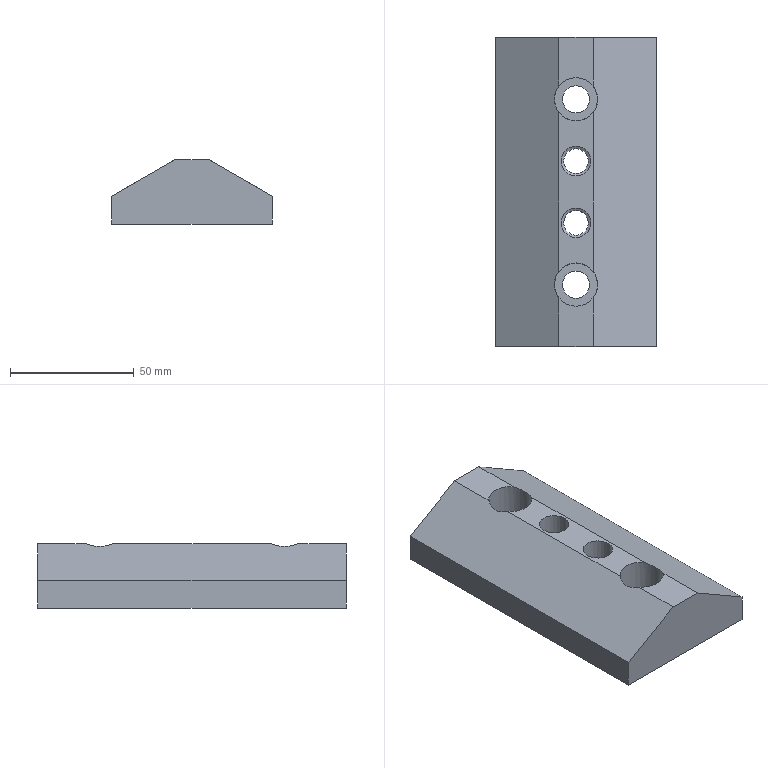Part | NX | features MAIN_BODY 2 | 1 solid | 22 faces | box 65 x 125 x 26 mm | volume 149619 mm3 | plane 12 | cylinder 8 | cone 2 | commonest cylinder face diameters 10 x2 11 x2 12 x2 17.5 x2
STEP:
#1=CARTESIAN_POINT('',(418.072,449.656,-244.));
#2=VERTEX_POINT('',#1);
#3=CARTESIAN_POINT('',(418.072,430.,-244.));
#4=VERTEX_POINT('',#3);
#5=CARTESIAN_POINT('',(418.072,555.,-244.));
#6=DIRECTION('',(0.,-1.,0.));
#7=VECTOR('',#6,1000.);
#8=LINE('',#5,#7);
#9=EDGE_CURVE('',#2,#4,#8,.T.);
#10=ORIENTED_EDGE('',*,*,#9,.T.);
#11=CARTESIAN_POINT('',(431.928,430.,-244.));
#12=VERTEX_POINT('',#11);
#13=CARTESIAN_POINT('',(392.5,430.,-244.));
#14=DIRECTION('',(1.,0.,0.));
#15=VECTOR('',#14,1000.);
#16=LINE('',#13,#15);
#17=EDGE_CURVE('',#4,#12,#16,.T.);
#18=ORIENTED_EDGE('',*,*,#17,.T.);
#19=CARTESIAN_POINT('',(431.928,449.656,-244.));
#20=VERTEX_POINT('',#19);
#21=CARTESIAN_POINT('',(431.928,555.,-244.));
#22=DIRECTION('',(0.,-1.,0.));
#23=VECTOR('',#22,1000.);
#24=LINE('',#21,#23);
#25=EDGE_CURVE('',#20,#12,#24,.T.);
#26=ORIENTED_EDGE('',*,*,#25,.F.);
#27=CARTESIAN_POINT('',(425.,455.,-244.));
#28=DIRECTION('',(0.,0.,-1.));
#29=DIRECTION('',(0.,-1.,0.));
#30=AXIS2_PLACEMENT_3D('',#27,#28,#29);
#31=CIRCLE('',#30,8.75);
#32=EDGE_CURVE('',#20,#2,#31,.T.);
#33=ORIENTED_EDGE('',*,*,#32,.T.);
#34=EDGE_LOOP('',(#10,#18,#26,#33));
#35=FACE_BOUND('',#34,.T.);
#36=CARTESIAN_POINT('',(392.5,430.,-244.));
#37=DIRECTION('',(0.,0.,-1.));
#38=DIRECTION('',(0.,-1.,0.));
#39=AXIS2_PLACEMENT_3D('',#36,#37,#38);
#40=PLANE('',#39);
#41=ADVANCED_FACE('',(#35),#40,.F.);
#42=CARTESIAN_POINT('',(418.072,524.656,-244.));
#43=VERTEX_POINT('',#42);
#44=CARTESIAN_POINT('',(418.072,460.344,-244.));
#45=VERTEX_POINT('',#44);
#46=CARTESIAN_POINT('',(418.072,555.,-244.));
#47=DIRECTION('',(0.,-1.,0.));
#48=VECTOR('',#47,1000.);
#49=LINE('',#46,#48);
#50=EDGE_CURVE('',#43,#45,#49,.T.);
#51=ORIENTED_EDGE('',*,*,#50,.T.);
#52=CARTESIAN_POINT('',(431.928,460.344,-244.));
#53=VERTEX_POINT('',#52);
#54=CARTESIAN_POINT('',(425.,455.,-244.));
#55=DIRECTION('',(0.,0.,-1.));
#56=DIRECTION('',(0.,-1.,0.));
#57=AXIS2_PLACEMENT_3D('',#54,#55,#56);
#58=CIRCLE('',#57,8.75);
#59=EDGE_CURVE('',#45,#53,#58,.T.);
#60=ORIENTED_EDGE('',*,*,#59,.T.);
#61=CARTESIAN_POINT('',(431.928,524.656,-244.));
#62=VERTEX_POINT('',#61);
#63=CARTESIAN_POINT('',(431.928,555.,-244.));
#64=DIRECTION('',(0.,-1.,0.));
#65=VECTOR('',#64,1000.);
#66=LINE('',#63,#65);
#67=EDGE_CURVE('',#62,#53,#66,.T.);
#68=ORIENTED_EDGE('',*,*,#67,.F.);
#69=CARTESIAN_POINT('',(425.,530.,-244.));
#70=DIRECTION('',(0.,0.,-1.));
#71=DIRECTION('',(0.,-1.,0.));
#72=AXIS2_PLACEMENT_3D('',#69,#70,#71);
#73=CIRCLE('',#72,8.75);
#74=EDGE_CURVE('',#62,#43,#73,.T.);
#75=ORIENTED_EDGE('',*,*,#74,.T.);
#76=EDGE_LOOP('',(#51,#60,#68,#75));
#77=FACE_BOUND('',#76,.T.);
#78=CARTESIAN_POINT('',(425.,474.,-244.));
#79=VERTEX_POINT('',#78);
#80=CARTESIAN_POINT('',(425.,480.,-244.));
#81=DIRECTION('',(0.,0.,-1.));
#82=DIRECTION('',(0.,-1.,0.));
#83=AXIS2_PLACEMENT_3D('',#80,#81,#82);
#84=CIRCLE('',#83,6.);
#85=EDGE_CURVE('',#79,#79,#84,.T.);
#86=ORIENTED_EDGE('',*,*,#85,.T.);
#87=EDGE_LOOP('',(#86));
#88=FACE_BOUND('',#87,.T.);
#89=CARTESIAN_POINT('',(425.,499.,-244.));
#90=VERTEX_POINT('',#89);
#91=CARTESIAN_POINT('',(425.,505.,-244.));
#92=DIRECTION('',(0.,0.,-1.));
#93=DIRECTION('',(0.,-1.,0.));
#94=AXIS2_PLACEMENT_3D('',#91,#92,#93);
#95=CIRCLE('',#94,6.);
#96=EDGE_CURVE('',#90,#90,#95,.T.);
#97=ORIENTED_EDGE('',*,*,#96,.T.);
#98=EDGE_LOOP('',(#97));
#99=FACE_BOUND('',#98,.T.);
#100=CARTESIAN_POINT('',(392.5,430.,-244.));
#101=DIRECTION('',(0.,0.,-1.));
#102=DIRECTION('',(0.,-1.,0.));
#103=AXIS2_PLACEMENT_3D('',#100,#101,#102);
#104=PLANE('',#103);
#105=ADVANCED_FACE('',(#77,#88,#99),#104,.F.);
#106=CARTESIAN_POINT('',(392.5,430.,-258.764));
#107=VERTEX_POINT('',#106);
#108=CARTESIAN_POINT('',(418.072,430.,-244.));
#109=DIRECTION('',(-0.866,0.,-0.5));
#110=VECTOR('',#109,1000.);
#111=LINE('',#108,#110);
#112=EDGE_CURVE('',#4,#107,#111,.T.);
#113=ORIENTED_EDGE('',*,*,#112,.T.);
#114=CARTESIAN_POINT('',(392.5,430.,-270.));
#115=VERTEX_POINT('',#114);
#116=CARTESIAN_POINT('',(392.5,430.,-244.));
#117=DIRECTION('',(0.,0.,-1.));
#118=VECTOR('',#117,1000.);
#119=LINE('',#116,#118);
#120=EDGE_CURVE('',#107,#115,#119,.T.);
#121=ORIENTED_EDGE('',*,*,#120,.T.);
#122=CARTESIAN_POINT('',(457.5,430.,-270.));
#123=VERTEX_POINT('',#122);
#124=CARTESIAN_POINT('',(392.5,430.,-270.));
#125=DIRECTION('',(1.,0.,0.));
#126=VECTOR('',#125,1000.);
#127=LINE('',#124,#126);
#128=EDGE_CURVE('',#115,#123,#127,.T.);
#129=ORIENTED_EDGE('',*,*,#128,.T.);
#130=CARTESIAN_POINT('',(457.5,430.,-258.764));
#131=VERTEX_POINT('',#130);
#132=CARTESIAN_POINT('',(457.5,430.,-244.));
#133=DIRECTION('',(0.,0.,-1.));
#134=VECTOR('',#133,1000.);
#135=LINE('',#132,#134);
#136=EDGE_CURVE('',#131,#123,#135,.T.);
#137=ORIENTED_EDGE('',*,*,#136,.F.);
#138=CARTESIAN_POINT('',(457.5,430.,-258.764));
#139=DIRECTION('',(-0.866,0.,0.5));
#140=VECTOR('',#139,1000.);
#141=LINE('',#138,#140);
#142=EDGE_CURVE('',#131,#12,#141,.T.);
#143=ORIENTED_EDGE('',*,*,#142,.T.);
#144=ORIENTED_EDGE('',*,*,#17,.F.);
#145=EDGE_LOOP('',(#113,#121,#129,#137,#143,#144));
#146=FACE_BOUND('',#145,.T.);
#147=CARTESIAN_POINT('',(392.5,430.,-244.));
#148=DIRECTION('',(0.,1.,0.));
#149=DIRECTION('',(-1.,0.,0.));
#150=AXIS2_PLACEMENT_3D('',#147,#148,#149);
#151=PLANE('',#150);
#152=ADVANCED_FACE('',(#146),#151,.F.);
#153=CARTESIAN_POINT('',(457.5,555.,-258.764));
#154=VERTEX_POINT('',#153);
#155=CARTESIAN_POINT('',(457.5,555.,-258.764));
#156=DIRECTION('',(0.,-1.,0.));
#157=VECTOR('',#156,1000.);
#158=LINE('',#155,#157);
#159=EDGE_CURVE('',#154,#131,#158,.T.);
#160=ORIENTED_EDGE('',*,*,#159,.T.);
#161=ORIENTED_EDGE('',*,*,#136,.T.);
#162=CARTESIAN_POINT('',(457.5,555.,-270.));
#163=VERTEX_POINT('',#162);
#164=CARTESIAN_POINT('',(457.5,430.,-270.));
#165=DIRECTION('',(0.,1.,0.));
#166=VECTOR('',#165,1000.);
#167=LINE('',#164,#166);
#168=EDGE_CURVE('',#123,#163,#167,.T.);
#169=ORIENTED_EDGE('',*,*,#168,.T.);
#170=CARTESIAN_POINT('',(457.5,555.,-244.));
#171=DIRECTION('',(0.,0.,-1.));
#172=VECTOR('',#171,1000.);
#173=LINE('',#170,#172);
#174=EDGE_CURVE('',#154,#163,#173,.T.);
#175=ORIENTED_EDGE('',*,*,#174,.F.);
#176=EDGE_LOOP('',(#160,#161,#169,#175));
#177=FACE_BOUND('',#176,.T.);
#178=CARTESIAN_POINT('',(457.5,430.,-244.));
#179=DIRECTION('',(-1.,0.,0.));
#180=DIRECTION('',(0.,0.,1.));
#181=AXIS2_PLACEMENT_3D('',#178,#179,#180);
#182=PLANE('',#181);
#183=ADVANCED_FACE('',(#177),#182,.F.);
#184=CARTESIAN_POINT('',(418.072,555.,-244.));
#185=VERTEX_POINT('',#184);
#186=CARTESIAN_POINT('',(392.5,555.,-258.764));
#187=VERTEX_POINT('',#186);
#188=CARTESIAN_POINT('',(418.072,555.,-244.));
#189=DIRECTION('',(-0.866,0.,-0.5));
#190=VECTOR('',#189,1000.);
#191=LINE('',#188,#190);
#192=EDGE_CURVE('',#185,#187,#191,.T.);
#193=ORIENTED_EDGE('',*,*,#192,.F.);
#194=CARTESIAN_POINT('',(431.928,555.,-244.));
#195=VERTEX_POINT('',#194);
#196=CARTESIAN_POINT('',(457.5,555.,-244.));
#197=DIRECTION('',(-1.,0.,0.));
#198=VECTOR('',#197,1000.);
#199=LINE('',#196,#198);
#200=EDGE_CURVE('',#195,#185,#199,.T.);
#201=ORIENTED_EDGE('',*,*,#200,.F.);
#202=CARTESIAN_POINT('',(457.5,555.,-258.764));
#203=DIRECTION('',(-0.866,0.,0.5));
#204=VECTOR('',#203,1000.);
#205=LINE('',#202,#204);
#206=EDGE_CURVE('',#154,#195,#205,.T.);
#207=ORIENTED_EDGE('',*,*,#206,.F.);
#208=ORIENTED_EDGE('',*,*,#174,.T.);
#209=CARTESIAN_POINT('',(392.5,555.,-270.));
#210=VERTEX_POINT('',#209);
#211=CARTESIAN_POINT('',(457.5,555.,-270.));
#212=DIRECTION('',(-1.,0.,0.));
#213=VECTOR('',#212,1000.);
#214=LINE('',#211,#213);
#215=EDGE_CURVE('',#163,#210,#214,.T.);
#216=ORIENTED_EDGE('',*,*,#215,.T.);
#217=CARTESIAN_POINT('',(392.5,555.,-244.));
#218=DIRECTION('',(0.,0.,-1.));
#219=VECTOR('',#218,1000.);
#220=LINE('',#217,#219);
#221=EDGE_CURVE('',#187,#210,#220,.T.);
#222=ORIENTED_EDGE('',*,*,#221,.F.);
#223=EDGE_LOOP('',(#193,#201,#207,#208,#216,#222));
#224=FACE_BOUND('',#223,.T.);
#225=CARTESIAN_POINT('',(457.5,555.,-244.));
#226=DIRECTION('',(0.,-1.,0.));
#227=DIRECTION('',(0.,0.,1.));
#228=AXIS2_PLACEMENT_3D('',#225,#226,#227);
#229=PLANE('',#228);
#230=ADVANCED_FACE('',(#224),#229,.F.);
#231=CARTESIAN_POINT('',(392.5,555.,-258.764));
#232=DIRECTION('',(0.,-1.,0.));
#233=VECTOR('',#232,1000.);
#234=LINE('',#231,#233);
#235=EDGE_CURVE('',#187,#107,#234,.T.);
#236=ORIENTED_EDGE('',*,*,#235,.F.);
#237=ORIENTED_EDGE('',*,*,#221,.T.);
#238=CARTESIAN_POINT('',(392.5,555.,-270.));
#239=DIRECTION('',(0.,-1.,0.));
#240=VECTOR('',#239,1000.);
#241=LINE('',#238,#240);
#242=EDGE_CURVE('',#210,#115,#241,.T.);
#243=ORIENTED_EDGE('',*,*,#242,.T.);
#244=ORIENTED_EDGE('',*,*,#120,.F.);
#245=EDGE_LOOP('',(#236,#237,#243,#244));
#246=FACE_BOUND('',#245,.T.);
#247=CARTESIAN_POINT('',(392.5,555.,-244.));
#248=DIRECTION('',(1.,0.,0.));
#249=DIRECTION('',(0.,1.,0.));
#250=AXIS2_PLACEMENT_3D('',#247,#248,#249);
#251=PLANE('',#250);
#252=ADVANCED_FACE('',(#246),#251,.F.);
#253=CARTESIAN_POINT('',(418.072,535.344,-244.));
#254=VERTEX_POINT('',#253);
#255=CARTESIAN_POINT('',(418.072,555.,-244.));
#256=DIRECTION('',(0.,-1.,0.));
#257=VECTOR('',#256,1000.);
#258=LINE('',#255,#257);
#259=EDGE_CURVE('',#185,#254,#258,.T.);
#260=ORIENTED_EDGE('',*,*,#259,.T.);
#261=CARTESIAN_POINT('',(431.928,535.344,-244.));
#262=VERTEX_POINT('',#261);
#263=CARTESIAN_POINT('',(425.,530.,-244.));
#264=DIRECTION('',(0.,0.,-1.));
#265=DIRECTION('',(0.,-1.,0.));
#266=AXIS2_PLACEMENT_3D('',#263,#264,#265);
#267=CIRCLE('',#266,8.75);
#268=EDGE_CURVE('',#254,#262,#267,.T.);
#269=ORIENTED_EDGE('',*,*,#268,.T.);
#270=CARTESIAN_POINT('',(431.928,555.,-244.));
#271=DIRECTION('',(0.,-1.,0.));
#272=VECTOR('',#271,1000.);
#273=LINE('',#270,#272);
#274=EDGE_CURVE('',#195,#262,#273,.T.);
#275=ORIENTED_EDGE('',*,*,#274,.F.);
#276=ORIENTED_EDGE('',*,*,#200,.T.);
#277=EDGE_LOOP('',(#260,#269,#275,#276));
#278=FACE_BOUND('',#277,.T.);
#279=CARTESIAN_POINT('',(392.5,430.,-244.));
#280=DIRECTION('',(0.,0.,-1.));
#281=DIRECTION('',(0.,-1.,0.));
#282=AXIS2_PLACEMENT_3D('',#279,#280,#281);
#283=PLANE('',#282);
#284=ADVANCED_FACE('',(#278),#283,.F.);
#285=CARTESIAN_POINT('',(425.,510.,-270.));
#286=VERTEX_POINT('',#285);
#287=CARTESIAN_POINT('',(425.,505.,-270.));
#288=DIRECTION('',(0.,0.,1.));
#289=DIRECTION('',(0.,1.,0.));
#290=AXIS2_PLACEMENT_3D('',#287,#288,#289);
#291=CIRCLE('',#290,5.);
#292=EDGE_CURVE('',#286,#286,#291,.T.);
#293=ORIENTED_EDGE('',*,*,#292,.T.);
#294=EDGE_LOOP('',(#293));
#295=FACE_BOUND('',#294,.T.);
#296=CARTESIAN_POINT('',(425.,485.,-270.));
#297=VERTEX_POINT('',#296);
#298=CARTESIAN_POINT('',(425.,480.,-270.));
#299=DIRECTION('',(0.,0.,1.));
#300=DIRECTION('',(0.,1.,0.));
#301=AXIS2_PLACEMENT_3D('',#298,#299,#300);
#302=CIRCLE('',#301,5.);
#303=EDGE_CURVE('',#297,#297,#302,.T.);
#304=ORIENTED_EDGE('',*,*,#303,.T.);
#305=EDGE_LOOP('',(#304));
#306=FACE_BOUND('',#305,.T.);
#307=CARTESIAN_POINT('',(425.,524.5,-270.));
#308=VERTEX_POINT('',#307);
#309=CARTESIAN_POINT('',(425.,530.,-270.));
#310=DIRECTION('',(0.,0.,-1.));
#311=DIRECTION('',(0.,-1.,0.));
#312=AXIS2_PLACEMENT_3D('',#309,#310,#311);
#313=CIRCLE('',#312,5.5);
#314=EDGE_CURVE('',#308,#308,#313,.T.);
#315=ORIENTED_EDGE('',*,*,#314,.F.);
#316=EDGE_LOOP('',(#315));
#317=FACE_BOUND('',#316,.T.);
#318=CARTESIAN_POINT('',(425.,449.5,-270.));
#319=VERTEX_POINT('',#318);
#320=CARTESIAN_POINT('',(425.,455.,-270.));
#321=DIRECTION('',(0.,0.,-1.));
#322=DIRECTION('',(0.,-1.,0.));
#323=AXIS2_PLACEMENT_3D('',#320,#321,#322);
#324=CIRCLE('',#323,5.5);
#325=EDGE_CURVE('',#319,#319,#324,.T.);
#326=ORIENTED_EDGE('',*,*,#325,.F.);
#327=EDGE_LOOP('',(#326));
#328=FACE_BOUND('',#327,.T.);
#329=ORIENTED_EDGE('',*,*,#128,.F.);
#330=ORIENTED_EDGE('',*,*,#242,.F.);
#331=ORIENTED_EDGE('',*,*,#215,.F.);
#332=ORIENTED_EDGE('',*,*,#168,.F.);
#333=EDGE_LOOP('',(#329,#330,#331,#332));
#334=FACE_BOUND('',#333,.T.);
#335=CARTESIAN_POINT('',(392.5,430.,-270.));
#336=DIRECTION('',(0.,0.,-1.));
#337=DIRECTION('',(0.,-1.,0.));
#338=AXIS2_PLACEMENT_3D('',#335,#336,#337);
#339=PLANE('',#338);
#340=ADVANCED_FACE('',(#295,#306,#317,#328,#334),#339,.T.);
#341=ORIENTED_EDGE('',*,*,#325,.T.);
#342=EDGE_LOOP('',(#341));
#343=FACE_BOUND('',#342,.T.);
#344=CARTESIAN_POINT('',(425.,449.5,-260.));
#345=VERTEX_POINT('',#344);
#346=CARTESIAN_POINT('',(425.,455.,-260.));
#347=DIRECTION('',(0.,0.,-1.));
#348=DIRECTION('',(0.,-1.,0.));
#349=AXIS2_PLACEMENT_3D('',#346,#347,#348);
#350=CIRCLE('',#349,5.5);
#351=EDGE_CURVE('',#345,#345,#350,.T.);
#352=ORIENTED_EDGE('',*,*,#351,.F.);
#353=EDGE_LOOP('',(#352));
#354=FACE_BOUND('',#353,.T.);
#355=CARTESIAN_POINT('',(425.,455.,-270.));
#356=DIRECTION('',(0.,0.,-1.));
#357=DIRECTION('',(0.,-1.,0.));
#358=AXIS2_PLACEMENT_3D('',#355,#356,#357);
#359=CYLINDRICAL_SURFACE('',#358,5.5);
#360=ADVANCED_FACE('',(#343,#354),#359,.F.);
#361=ORIENTED_EDGE('',*,*,#351,.T.);
#362=EDGE_LOOP('',(#361));
#363=FACE_BOUND('',#362,.T.);
#364=CARTESIAN_POINT('',(425.,446.25,-260.));
#365=VERTEX_POINT('',#364);
#366=CARTESIAN_POINT('',(425.,455.,-260.));
#367=DIRECTION('',(0.,0.,-1.));
#368=DIRECTION('',(0.,-1.,0.));
#369=AXIS2_PLACEMENT_3D('',#366,#367,#368);
#370=CIRCLE('',#369,8.75);
#371=EDGE_CURVE('',#365,#365,#370,.T.);
#372=ORIENTED_EDGE('',*,*,#371,.F.);
#373=EDGE_LOOP('',(#372));
#374=FACE_BOUND('',#373,.T.);
#375=CARTESIAN_POINT('',(425.,455.,-260.));
#376=DIRECTION('',(0.,0.,-1.));
#377=DIRECTION('',(0.,-1.,0.));
#378=AXIS2_PLACEMENT_3D('',#375,#376,#377);
#379=PLANE('',#378);
#380=ADVANCED_FACE('',(#363,#374),#379,.F.);
#381=CARTESIAN_POINT('',(425.,455.,-240.));
#382=DIRECTION('',(-0.5,0.,0.866));
#383=DIRECTION('',(-0.866,0.,-0.5));
#384=AXIS2_PLACEMENT_3D('',#381,#382,#383);
#385=ELLIPSE('',#384,10.104,8.75);
#386=EDGE_CURVE('',#2,#45,#385,.F.);
#387=ORIENTED_EDGE('',*,*,#386,.F.);
#388=ORIENTED_EDGE('',*,*,#32,.F.);
#389=CARTESIAN_POINT('',(425.,455.,-240.));
#390=DIRECTION('',(0.5,0.,0.866));
#391=DIRECTION('',(0.866,0.,-0.5));
#392=AXIS2_PLACEMENT_3D('',#389,#390,#391);
#393=ELLIPSE('',#392,10.104,8.75);
#394=EDGE_CURVE('',#53,#20,#393,.F.);
#395=ORIENTED_EDGE('',*,*,#394,.F.);
#396=ORIENTED_EDGE('',*,*,#59,.F.);
#397=EDGE_LOOP('',(#387,#388,#395,#396));
#398=FACE_BOUND('',#397,.T.);
#399=ORIENTED_EDGE('',*,*,#371,.T.);
#400=EDGE_LOOP('',(#399));
#401=FACE_BOUND('',#400,.T.);
#402=CARTESIAN_POINT('',(425.,455.,-244.));
#403=DIRECTION('',(0.,0.,-1.));
#404=DIRECTION('',(0.,-1.,0.));
#405=AXIS2_PLACEMENT_3D('',#402,#403,#404);
#406=CYLINDRICAL_SURFACE('',#405,8.75);
#407=ADVANCED_FACE('',(#398,#401),#406,.F.);
#408=ORIENTED_EDGE('',*,*,#314,.T.);
#409=EDGE_LOOP('',(#408));
#410=FACE_BOUND('',#409,.T.);
#411=CARTESIAN_POINT('',(425.,524.5,-260.));
#412=VERTEX_POINT('',#411);
#413=CARTESIAN_POINT('',(425.,530.,-260.));
#414=DIRECTION('',(0.,0.,-1.));
#415=DIRECTION('',(0.,-1.,0.));
#416=AXIS2_PLACEMENT_3D('',#413,#414,#415);
#417=CIRCLE('',#416,5.5);
#418=EDGE_CURVE('',#412,#412,#417,.T.);
#419=ORIENTED_EDGE('',*,*,#418,.F.);
#420=EDGE_LOOP('',(#419));
#421=FACE_BOUND('',#420,.T.);
#422=CARTESIAN_POINT('',(425.,530.,-270.));
#423=DIRECTION('',(0.,0.,-1.));
#424=DIRECTION('',(0.,-1.,0.));
#425=AXIS2_PLACEMENT_3D('',#422,#423,#424);
#426=CYLINDRICAL_SURFACE('',#425,5.5);
#427=ADVANCED_FACE('',(#410,#421),#426,.F.);
#428=ORIENTED_EDGE('',*,*,#418,.T.);
#429=EDGE_LOOP('',(#428));
#430=FACE_BOUND('',#429,.T.);
#431=CARTESIAN_POINT('',(425.,521.25,-260.));
#432=VERTEX_POINT('',#431);
#433=CARTESIAN_POINT('',(425.,530.,-260.));
#434=DIRECTION('',(0.,0.,-1.));
#435=DIRECTION('',(0.,-1.,0.));
#436=AXIS2_PLACEMENT_3D('',#433,#434,#435);
#437=CIRCLE('',#436,8.75);
#438=EDGE_CURVE('',#432,#432,#437,.T.);
#439=ORIENTED_EDGE('',*,*,#438,.F.);
#440=EDGE_LOOP('',(#439));
#441=FACE_BOUND('',#440,.T.);
#442=CARTESIAN_POINT('',(425.,530.,-260.));
#443=DIRECTION('',(0.,0.,-1.));
#444=DIRECTION('',(0.,-1.,0.));
#445=AXIS2_PLACEMENT_3D('',#442,#443,#444);
#446=PLANE('',#445);
#447=ADVANCED_FACE('',(#430,#441),#446,.F.);
#448=CARTESIAN_POINT('',(425.,530.,-240.));
#449=DIRECTION('',(-0.5,0.,0.866));
#450=DIRECTION('',(-0.866,0.,-0.5));
#451=AXIS2_PLACEMENT_3D('',#448,#449,#450);
#452=ELLIPSE('',#451,10.104,8.75);
#453=EDGE_CURVE('',#43,#254,#452,.F.);
#454=ORIENTED_EDGE('',*,*,#453,.F.);
#455=ORIENTED_EDGE('',*,*,#74,.F.);
#456=CARTESIAN_POINT('',(425.,530.,-240.));
#457=DIRECTION('',(0.5,0.,0.866));
#458=DIRECTION('',(0.866,0.,-0.5));
#459=AXIS2_PLACEMENT_3D('',#456,#457,#458);
#460=ELLIPSE('',#459,10.104,8.75);
#461=EDGE_CURVE('',#262,#62,#460,.F.);
#462=ORIENTED_EDGE('',*,*,#461,.F.);
#463=ORIENTED_EDGE('',*,*,#268,.F.);
#464=EDGE_LOOP('',(#454,#455,#462,#463));
#465=FACE_BOUND('',#464,.T.);
#466=ORIENTED_EDGE('',*,*,#438,.T.);
#467=EDGE_LOOP('',(#466));
#468=FACE_BOUND('',#467,.T.);
#469=CARTESIAN_POINT('',(425.,530.,-244.));
#470=DIRECTION('',(0.,0.,-1.));
#471=DIRECTION('',(0.,-1.,0.));
#472=AXIS2_PLACEMENT_3D('',#469,#470,#471);
#473=CYLINDRICAL_SURFACE('',#472,8.75);
#474=ADVANCED_FACE('',(#465,#468),#473,.F.);
#475=CARTESIAN_POINT('',(425.,485.,-255.577));
#476=VERTEX_POINT('',#475);
#477=CARTESIAN_POINT('',(425.,480.,-255.577));
#478=DIRECTION('',(0.,0.,1.));
#479=DIRECTION('',(0.,1.,0.));
#480=AXIS2_PLACEMENT_3D('',#477,#478,#479);
#481=CIRCLE('',#480,5.);
#482=EDGE_CURVE('',#476,#476,#481,.F.);
#483=ORIENTED_EDGE('',*,*,#482,.T.);
#484=EDGE_LOOP('',(#483));
#485=FACE_BOUND('',#484,.T.);
#486=CARTESIAN_POINT('',(425.,474.,-255.));
#487=VERTEX_POINT('',#486);
#488=CARTESIAN_POINT('',(425.,480.,-255.));
#489=DIRECTION('',(0.,0.,-1.));
#490=DIRECTION('',(0.,-1.,0.));
#491=AXIS2_PLACEMENT_3D('',#488,#489,#490);
#492=CIRCLE('',#491,6.);
#493=EDGE_CURVE('',#487,#487,#492,.T.);
#494=ORIENTED_EDGE('',*,*,#493,.F.);
#495=EDGE_LOOP('',(#494));
#496=FACE_BOUND('',#495,.T.);
#497=CARTESIAN_POINT('',(425.,480.,-255.));
#498=DIRECTION('',(0.,0.,1.));
#499=DIRECTION('',(0.,1.,0.));
#500=AXIS2_PLACEMENT_3D('',#497,#498,#499);
#501=CONICAL_SURFACE('',#500,6.,1.047);
#502=ADVANCED_FACE('',(#485,#496),#501,.F.);
#503=ORIENTED_EDGE('',*,*,#493,.T.);
#504=EDGE_LOOP('',(#503));
#505=FACE_BOUND('',#504,.T.);
#506=ORIENTED_EDGE('',*,*,#85,.F.);
#507=EDGE_LOOP('',(#506));
#508=FACE_BOUND('',#507,.T.);
#509=CARTESIAN_POINT('',(425.,480.,-244.));
#510=DIRECTION('',(0.,0.,-1.));
#511=DIRECTION('',(0.,-1.,0.));
#512=AXIS2_PLACEMENT_3D('',#509,#510,#511);
#513=CYLINDRICAL_SURFACE('',#512,6.);
#514=ADVANCED_FACE('',(#505,#508),#513,.F.);
#515=CARTESIAN_POINT('',(425.,510.,-255.577));
#516=VERTEX_POINT('',#515);
#517=CARTESIAN_POINT('',(425.,505.,-255.577));
#518=DIRECTION('',(0.,0.,1.));
#519=DIRECTION('',(0.,1.,0.));
#520=AXIS2_PLACEMENT_3D('',#517,#518,#519);
#521=CIRCLE('',#520,5.);
#522=EDGE_CURVE('',#516,#516,#521,.F.);
#523=ORIENTED_EDGE('',*,*,#522,.T.);
#524=EDGE_LOOP('',(#523));
#525=FACE_BOUND('',#524,.T.);
#526=CARTESIAN_POINT('',(425.,499.,-255.));
#527=VERTEX_POINT('',#526);
#528=CARTESIAN_POINT('',(425.,505.,-255.));
#529=DIRECTION('',(0.,0.,-1.));
#530=DIRECTION('',(0.,-1.,0.));
#531=AXIS2_PLACEMENT_3D('',#528,#529,#530);
#532=CIRCLE('',#531,6.);
#533=EDGE_CURVE('',#527,#527,#532,.T.);
#534=ORIENTED_EDGE('',*,*,#533,.F.);
#535=EDGE_LOOP('',(#534));
#536=FACE_BOUND('',#535,.T.);
#537=CARTESIAN_POINT('',(425.,505.,-255.));
#538=DIRECTION('',(0.,0.,1.));
#539=DIRECTION('',(0.,1.,0.));
#540=AXIS2_PLACEMENT_3D('',#537,#538,#539);
#541=CONICAL_SURFACE('',#540,6.,1.047);
#542=ADVANCED_FACE('',(#525,#536),#541,.F.);
#543=ORIENTED_EDGE('',*,*,#533,.T.);
#544=EDGE_LOOP('',(#543));
#545=FACE_BOUND('',#544,.T.);
#546=ORIENTED_EDGE('',*,*,#96,.F.);
#547=EDGE_LOOP('',(#546));
#548=FACE_BOUND('',#547,.T.);
#549=CARTESIAN_POINT('',(425.,505.,-244.));
#550=DIRECTION('',(0.,0.,-1.));
#551=DIRECTION('',(0.,-1.,0.));
#552=AXIS2_PLACEMENT_3D('',#549,#550,#551);
#553=CYLINDRICAL_SURFACE('',#552,6.);
#554=ADVANCED_FACE('',(#545,#548),#553,.F.);
#555=ORIENTED_EDGE('',*,*,#303,.F.);
#556=EDGE_LOOP('',(#555));
#557=FACE_BOUND('',#556,.T.);
#558=ORIENTED_EDGE('',*,*,#482,.F.);
#559=EDGE_LOOP('',(#558));
#560=FACE_BOUND('',#559,.T.);
#561=CARTESIAN_POINT('',(425.,480.,-270.));
#562=DIRECTION('',(0.,0.,1.));
#563=DIRECTION('',(0.,1.,0.));
#564=AXIS2_PLACEMENT_3D('',#561,#562,#563);
#565=CYLINDRICAL_SURFACE('',#564,5.);
#566=ADVANCED_FACE('',(#557,#560),#565,.F.);
#567=ORIENTED_EDGE('',*,*,#292,.F.);
#568=EDGE_LOOP('',(#567));
#569=FACE_BOUND('',#568,.T.);
#570=ORIENTED_EDGE('',*,*,#522,.F.);
#571=EDGE_LOOP('',(#570));
#572=FACE_BOUND('',#571,.T.);
#573=CARTESIAN_POINT('',(425.,505.,-270.));
#574=DIRECTION('',(0.,0.,1.));
#575=DIRECTION('',(0.,1.,0.));
#576=AXIS2_PLACEMENT_3D('',#573,#574,#575);
#577=CYLINDRICAL_SURFACE('',#576,5.);
#578=ADVANCED_FACE('',(#569,#572),#577,.F.);
#579=ORIENTED_EDGE('',*,*,#67,.T.);
#580=ORIENTED_EDGE('',*,*,#394,.T.);
#581=ORIENTED_EDGE('',*,*,#25,.T.);
#582=ORIENTED_EDGE('',*,*,#142,.F.);
#583=ORIENTED_EDGE('',*,*,#159,.F.);
#584=ORIENTED_EDGE('',*,*,#206,.T.);
#585=ORIENTED_EDGE('',*,*,#274,.T.);
#586=ORIENTED_EDGE('',*,*,#461,.T.);
#587=EDGE_LOOP('',(#579,#580,#581,#582,#583,#584,#585,#586));
#588=FACE_BOUND('',#587,.T.);
#589=CARTESIAN_POINT('',(457.5,555.,-258.764));
#590=DIRECTION('',(0.5,0.,0.866));
#591=DIRECTION('',(0.866,0.,-0.5));
#592=AXIS2_PLACEMENT_3D('',#589,#590,#591);
#593=PLANE('',#592);
#594=ADVANCED_FACE('',(#588),#593,.T.);
#595=ORIENTED_EDGE('',*,*,#9,.F.);
#596=ORIENTED_EDGE('',*,*,#386,.T.);
#597=ORIENTED_EDGE('',*,*,#50,.F.);
#598=ORIENTED_EDGE('',*,*,#453,.T.);
#599=ORIENTED_EDGE('',*,*,#259,.F.);
#600=ORIENTED_EDGE('',*,*,#192,.T.);
#601=ORIENTED_EDGE('',*,*,#235,.T.);
#602=ORIENTED_EDGE('',*,*,#112,.F.);
#603=EDGE_LOOP('',(#595,#596,#597,#598,#599,#600,#601,#602));
#604=FACE_BOUND('',#603,.T.);
#605=CARTESIAN_POINT('',(418.072,555.,-244.));
#606=DIRECTION('',(-0.5,0.,0.866));
#607=DIRECTION('',(0.866,0.,0.5));
#608=AXIS2_PLACEMENT_3D('',#605,#606,#607);
#609=PLANE('',#608);
#610=ADVANCED_FACE('',(#604),#609,.T.);
#611=CLOSED_SHELL('',(#41,#105,#152,#183,#230,#252,#284,#340,#360,#380,#407,#427,#447,#474,#502,#514,#542,#554,#566,#578,#594,#610));
#612=MANIFOLD_SOLID_BREP('',#611);
#613=(LENGTH_UNIT()NAMED_UNIT(*)SI_UNIT(.MILLI.,.METRE.));
#614=UNCERTAINTY_MEASURE_WITH_UNIT(LENGTH_MEASURE(0.00001),#613,'','');
#615=(NAMED_UNIT(*)PLANE_ANGLE_UNIT()SI_UNIT($,.RADIAN.));
#616=(NAMED_UNIT(*)SI_UNIT($,.STERADIAN.)SOLID_ANGLE_UNIT());
#617=(GEOMETRIC_REPRESENTATION_CONTEXT(3)GLOBAL_UNCERTAINTY_ASSIGNED_CONTEXT((#614))GLOBAL_UNIT_ASSIGNED_CONTEXT((#613,#615,#616))REPRESENTATION_CONTEXT('',''));
#618=ADVANCED_BREP_SHAPE_REPRESENTATION('',(#612),#617);